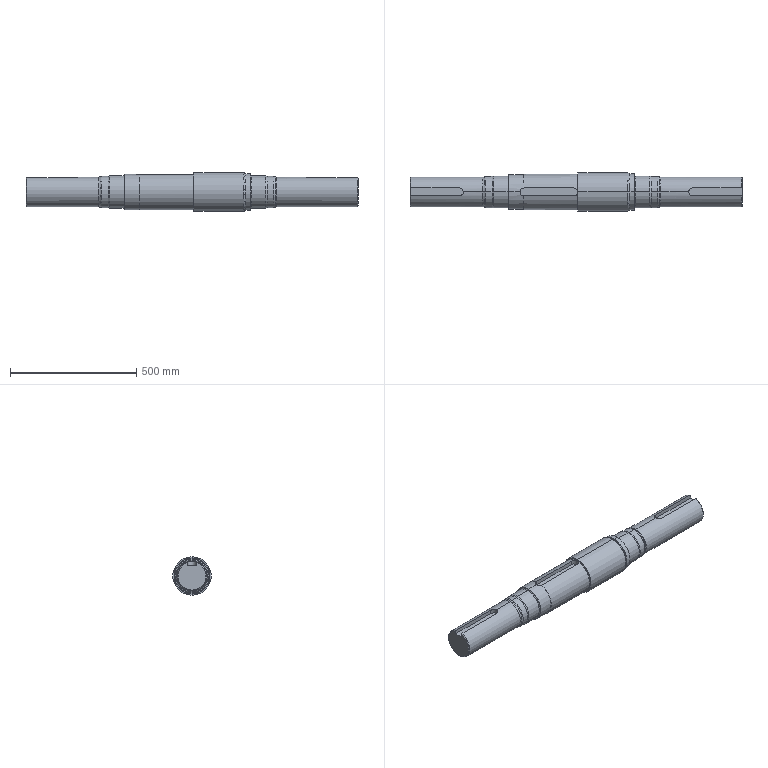Part | SolidWorks | features Fillet 2, ICE 2, Chamfer 1, Revolution 1 | 1 solid | 67 faces | box 1314 x 152.146 x 152.146 mm | volume 17037047 mm3 | cylinder 26 | torus 18 | plane 14 | cone 9 | commonest cylinder face diameters 31.75 x6 117.475 x4 123.825 x4 127.038 x4 139.395 x2 139.725 x2